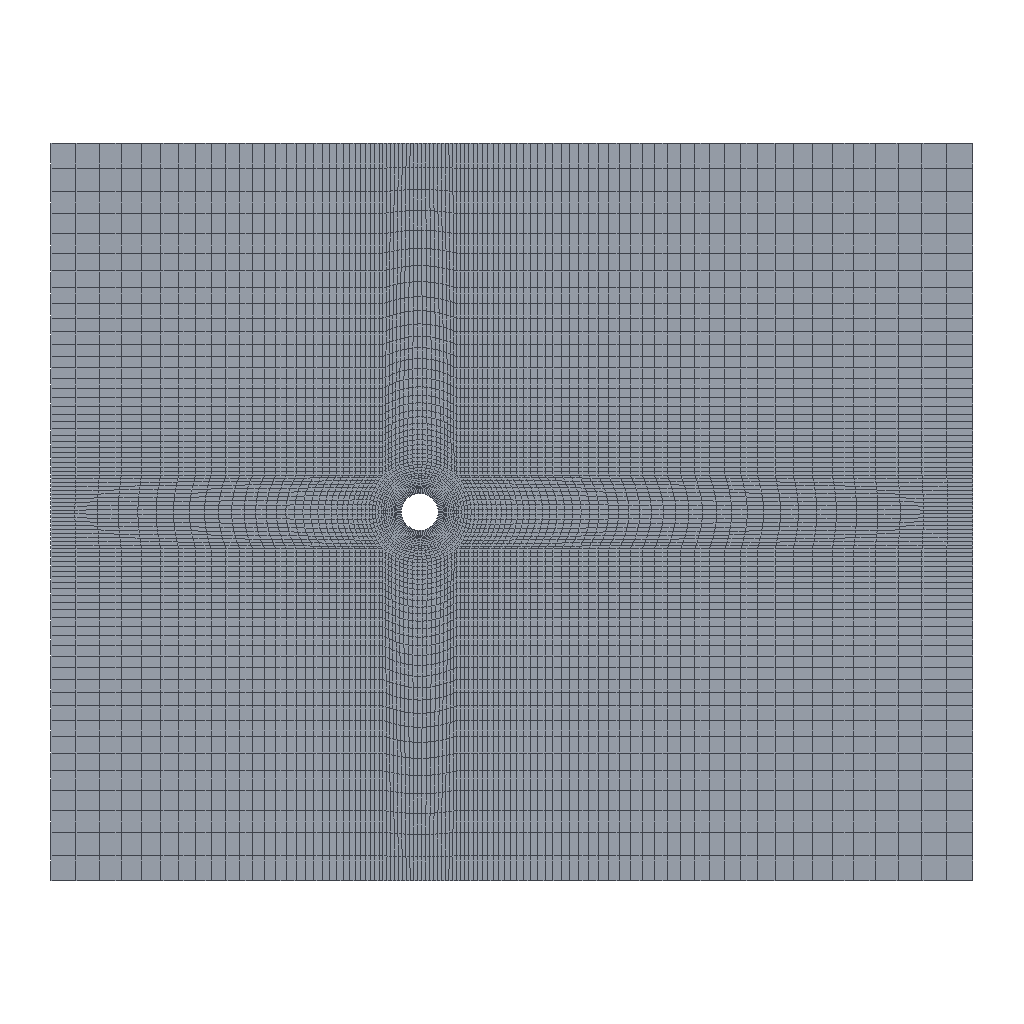Simulation study | ansys fluent
Set-up summary:
category,name,step,type,value,unit,region
solver,ansys_fluent,,Fluent 26.1.0
units,SI m-kg-s (Fluent internal),,stated,boundary values in the units shown in brackets; results in listed units
analysis,deck-1.cas,,cfd steady,"dimension=2D; solver=2d, dp, pbns, lam (2d, double precision, pressure-based, laminar); source_case=2.cas"
model,Space,deck-1.cas,,2D
model,Time,deck-1.cas,,Steady
model,Viscous,deck-1.cas,,Laminar
model,Heat Transfer,deck-1.cas,,Disabled
model,Multiphase,deck-1.cas,,Disabled
analysis,deck-2.cas,,"cfd unsteady, 2nd-order implicit","dimension=2D; solver=2d, dp, pbns, lam, transient (2d, double precision, pressure-based, laminar, transient); source_case=4.cas"
model,Space,deck-2.cas,,2D
model,Time,deck-2.cas,,"Unsteady, 2nd-Order Implicit"
model,Viscous,deck-2.cas,,Laminar
model,Heat Transfer,deck-2.cas,,Disabled
model,Multiphase,deck-2.cas,,Disabled
analysis,deck-3.cas,,"cfd unsteady, 2nd-order implicit","dimension=2D; solver=2d, dp, pbns, lam, transient (2d, double precision, pressure-based, laminar, transient); source_case=5.cas.h5"
model,Space,deck-3.cas,,2D
model,Time,deck-3.cas,,"Unsteady, 2nd-Order Implicit"
model,Viscous,deck-3.cas,,Laminar
model,Heat Transfer,deck-3.cas,,Disabled
model,Multiphase,deck-3.cas,,Disabled
analysis,deck-4.cas,,cfd steady,"dimension=2D; solver=2d, dp, pbns, lam (2d, double precision, pressure-based, laminar); source_case=.cas.h5"
model,Space,deck-4.cas,,2D
model,Time,deck-4.cas,,Steady
model,Viscous,deck-4.cas,,Laminar
model,Heat Transfer,deck-4.cas,,Disabled
model,Multiphase,deck-4.cas,,Disabled
mesh,deck-1.cas,,nodes,8374
mesh,deck-1.cas,,elements,8167
mesh,deck-1.cas,,faces,16541
mesh,deck-1.cas,,note,elements = cells; counts from the case file zone headers
mesh,deck-2.cas,,nodes,8374
mesh,deck-2.cas,,elements,8167
mesh,deck-2.cas,,faces,16541
mesh,deck-2.cas,,note,elements = cells; counts from the case file zone headers
mesh,deck-3.cas,,nodes,8374
mesh,deck-3.cas,,elements,8167
mesh,deck-3.cas,,faces,16541
mesh,deck-3.cas,,note,elements = cells; counts from the case file zone headers
mesh,deck-4.cas,,nodes,8374
mesh,deck-4.cas,,elements,8167
mesh,deck-4.cas,,faces,16541
mesh,deck-4.cas,,note,elements = cells; counts from the case file zone headers
cell_zone,fluid,deck-1.cas,fluid,material=air,,zone 2
cell_zone,fluid,deck-2.cas,fluid,material=air,,zone 2
cell_zone,fluid,deck-3.cas,fluid,material=air,,zone 2
cell_zone,fluid,deck-4.cas,fluid,material=air,,zone 2
material,air (fluid),,Density,1,kg/m^3
material,air (fluid),,Viscosity,0.01,kg/(m s)
material,aluminum (solid),,Density,2719,kg/m^3
bc,out,deck-1.cas,pressure-outlet,,,zone 3
bc,in,deck-1.cas,velocity-inlet,Velocity Magnitude [m/s]=1,,zone 4
bc,sym2,deck-1.cas,symmetry,,,zone 5
bc,sym1,deck-1.cas,symmetry,,,zone 6
bc,cylinder,deck-1.cas,wall,Wall Motion=Stationary Wall; Shear Boundary Condition=No Slip,,zone 7
bc,out,deck-2.cas,pressure-outlet,,,zone 3
bc,in,deck-2.cas,velocity-inlet,Velocity Magnitude [m/s]=1,,zone 4
bc,sym2,deck-2.cas,symmetry,,,zone 5
bc,sym1,deck-2.cas,symmetry,,,zone 6
bc,cylinder,deck-2.cas,wall,Wall Motion=Stationary Wall; Shear Boundary Condition=No Slip,,zone 7
bc,out,deck-3.cas,pressure-outlet,,,zone 3
bc,in,deck-3.cas,velocity-inlet,Velocity Magnitude [m/s]=1,,zone 4
bc,sym2,deck-3.cas,symmetry,,,zone 5
bc,sym1,deck-3.cas,symmetry,,,zone 6
bc,cylinder,deck-3.cas,wall,Wall Motion=Stationary Wall; Shear Boundary Condition=No Slip,,zone 7
bc,out,deck-4.cas,pressure-outlet,,,zone 3
bc,in,deck-4.cas,velocity-inlet,Velocity Magnitude [m/s]=1,,zone 4
bc,sym2,deck-4.cas,symmetry,,,zone 5
bc,sym1,deck-4.cas,symmetry,,,zone 6
bc,cylinder,deck-4.cas,wall,Wall Motion=Stationary Wall; Shear Boundary Condition=No Slip,,zone 7
Results summary:
result,mass flow rate cylinder,deck-1.cas,,-0,kg/s
result,mass flow rate in,deck-1.cas,,20,kg/s
result,mass flow rate out,deck-1.cas,,-20.002,kg/s
result,mass flow rate Net,deck-1.cas,,-0.00166,kg/s
result,wall force total cylinder,deck-1.cas,,"(0.5968, 0.006984, 0)",N
result,wall force pressure cylinder,deck-1.cas,,"(0.438, 0.005052, 0)",N
result,wall force viscous cylinder,deck-1.cas,,"(0.1588, 0.001932, 0)",N
result,wall force total Net,deck-1.cas,,"(0.5968, 0.006984, 0)",N
result,wall force pressure Net,deck-1.cas,,"(0.438, 0.005052, 0)",N
result,wall force viscous Net,deck-1.cas,,"(0.1588, 0.001932, 0)",N
result,mass flow rate cylinder,deck-2.cas,,-0,kg/s
result,mass flow rate in,deck-2.cas,,20,kg/s
result,mass flow rate out,deck-2.cas,,-20,kg/s
result,mass flow rate Net,deck-2.cas,,5.96046e-08,kg/s
result,wall force total cylinder,deck-2.cas,,"(0.6818, 0.1464, 0)",N
result,wall force pressure cylinder,deck-2.cas,,"(0.5051, 0.1305, 0)",N
result,wall force viscous cylinder,deck-2.cas,,"(0.1767, 0.01586, 0)",N
result,wall force total Net,deck-2.cas,,"(0.6818, 0.1464, 0)",N
result,wall force pressure Net,deck-2.cas,,"(0.5051, 0.1305, 0)",N
result,wall force viscous Net,deck-2.cas,,"(0.1767, 0.01586, 0)",N
result,mass flow rate cylinder,deck-3.cas,,-0,kg/s
result,mass flow rate in,deck-3.cas,,20,kg/s
result,mass flow rate out,deck-3.cas,,-20,kg/s
result,mass flow rate Net,deck-3.cas,,5.96046e-08,kg/s
result,wall force total cylinder,deck-3.cas,,"(0.6818, 0.1464, 0)",N
result,wall force pressure cylinder,deck-3.cas,,"(0.5051, 0.1305, 0)",N
result,wall force viscous cylinder,deck-3.cas,,"(0.1767, 0.01586, 0)",N
result,wall force total Net,deck-3.cas,,"(0.6818, 0.1464, 0)",N
result,wall force pressure Net,deck-3.cas,,"(0.5051, 0.1305, 0)",N
result,wall force viscous Net,deck-3.cas,,"(0.1767, 0.01586, 0)",N
result,mass flow rate cylinder,deck-4.cas,,-0,kg/s
result,mass flow rate in,deck-4.cas,,20,kg/s
result,mass flow rate out,deck-4.cas,,-20.002,kg/s
result,mass flow rate Net,deck-4.cas,,-0.00166,kg/s
result,wall force total cylinder,deck-4.cas,,"(0.5968, 0.006984, 0)",N
result,wall force pressure cylinder,deck-4.cas,,"(0.438, 0.005052, 0)",N
result,wall force viscous cylinder,deck-4.cas,,"(0.1588, 0.001932, 0)",N
result,wall force total Net,deck-4.cas,,"(0.5968, 0.006984, 0)",N
result,wall force pressure Net,deck-4.cas,,"(0.438, 0.005052, 0)",N
result,wall force viscous Net,deck-4.cas,,"(0.1588, 0.001932, 0)",N